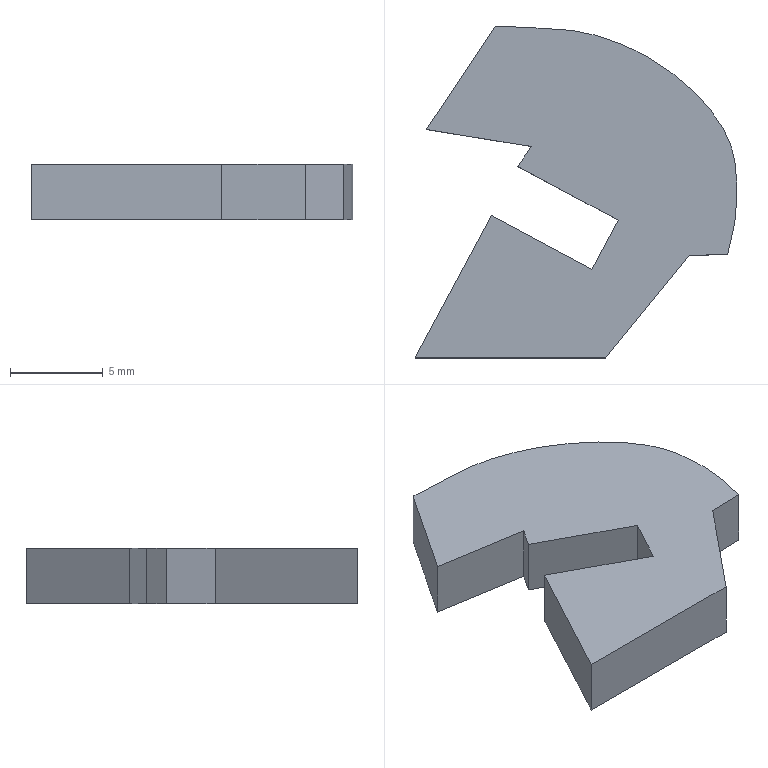Part | SolidWorks | features BaseBody 1 | 1 solid | 17 faces | box 17.352 x 17.888 x 3 mm | volume 573.183 mm3 | plane 13 | spline 4
STEP:
#1=CARTESIAN_POINT('',(42.678,-11.276,-1.5));
#2=VERTEX_POINT('',#1);
#3=CARTESIAN_POINT('',(42.678,-11.276,-1.5));
#4=VERTEX_POINT('',#3);
#5=CARTESIAN_POINT('',(42.678,-11.276,-1.5));
#6=CARTESIAN_POINT('',(42.678,-11.276,-1.5));
#7=CARTESIAN_POINT('',(42.678,-11.276,-1.5));
#8=CARTESIAN_POINT('',(42.678,-11.276,-1.5));
#9=B_SPLINE_CURVE_WITH_KNOTS('',3,(#5,#6,#7,#8),.UNSPECIFIED.,.F.,.F.,(4,4),(0.,0.000000418),.UNSPECIFIED.);
#10=EDGE_CURVE('',#2,#4,#9,.T.);
#11=ORIENTED_EDGE('',*,*,#10,.F.);
#12=CARTESIAN_POINT('',(40.608,-11.347,-1.5));
#13=VERTEX_POINT('',#12);
#14=CARTESIAN_POINT('',(42.678,-11.276,-1.5));
#15=DIRECTION('',(0.9994,0.03426,0.));
#16=VECTOR('',#15,1000.);
#17=LINE('',#14,#16);
#18=EDGE_CURVE('',#13,#2,#17,.T.);
#19=ORIENTED_EDGE('',*,*,#18,.F.);
#20=CARTESIAN_POINT('',(36.112,-16.862,-1.5));
#21=VERTEX_POINT('',#20);
#22=CARTESIAN_POINT('',(40.608,-11.347,-1.5));
#23=DIRECTION('',(0.6319,0.775,0.));
#24=VECTOR('',#23,1000.);
#25=LINE('',#22,#24);
#26=EDGE_CURVE('',#21,#13,#25,.T.);
#27=ORIENTED_EDGE('',*,*,#26,.F.);
#28=CARTESIAN_POINT('',(25.831,-16.862,-1.5));
#29=VERTEX_POINT('',#28);
#30=CARTESIAN_POINT('',(36.112,-16.862,-1.5));
#31=DIRECTION('',(1.,0.,0.));
#32=VECTOR('',#31,1000.);
#33=LINE('',#30,#32);
#34=EDGE_CURVE('',#29,#21,#33,.T.);
#35=ORIENTED_EDGE('',*,*,#34,.F.);
#36=CARTESIAN_POINT('',(29.948,-9.183,-1.5));
#37=VERTEX_POINT('',#36);
#38=CARTESIAN_POINT('',(25.831,-16.862,-1.5));
#39=DIRECTION('',(-0.4726,-0.8813,0.));
#40=VECTOR('',#39,1000.);
#41=LINE('',#38,#40);
#42=EDGE_CURVE('',#37,#29,#41,.T.);
#43=ORIENTED_EDGE('',*,*,#42,.F.);
#44=CARTESIAN_POINT('',(35.355,-12.082,-1.5));
#45=VERTEX_POINT('',#44);
#46=CARTESIAN_POINT('',(29.948,-9.183,-1.5));
#47=DIRECTION('',(-0.8814,0.4725,0.));
#48=VECTOR('',#47,1000.);
#49=LINE('',#46,#48);
#50=EDGE_CURVE('',#45,#37,#49,.T.);
#51=ORIENTED_EDGE('',*,*,#50,.F.);
#52=CARTESIAN_POINT('',(36.773,-9.438,-1.5));
#53=VERTEX_POINT('',#52);
#54=CARTESIAN_POINT('',(35.355,-12.082,-1.5));
#55=DIRECTION('',(-0.4725,-0.8814,0.));
#56=VECTOR('',#55,1000.);
#57=LINE('',#54,#56);
#58=EDGE_CURVE('',#53,#45,#57,.T.);
#59=ORIENTED_EDGE('',*,*,#58,.F.);
#60=CARTESIAN_POINT('',(31.367,-6.54,-1.5));
#61=VERTEX_POINT('',#60);
#62=CARTESIAN_POINT('',(36.773,-9.438,-1.5));
#63=DIRECTION('',(0.8814,-0.4725,0.));
#64=VECTOR('',#63,1000.);
#65=LINE('',#62,#64);
#66=EDGE_CURVE('',#61,#53,#65,.T.);
#67=ORIENTED_EDGE('',*,*,#66,.F.);
#68=CARTESIAN_POINT('',(32.093,-5.467,-1.5));
#69=VERTEX_POINT('',#68);
#70=CARTESIAN_POINT('',(31.367,-6.54,-1.5));
#71=DIRECTION('',(-0.5603,-0.8283,0.));
#72=VECTOR('',#71,1000.);
#73=LINE('',#70,#72);
#74=EDGE_CURVE('',#69,#61,#73,.T.);
#75=ORIENTED_EDGE('',*,*,#74,.F.);
#76=CARTESIAN_POINT('',(26.438,-4.552,-1.5));
#77=VERTEX_POINT('',#76);
#78=CARTESIAN_POINT('',(32.093,-5.467,-1.5));
#79=DIRECTION('',(0.9872,-0.1597,0.));
#80=VECTOR('',#79,1000.);
#81=LINE('',#78,#80);
#82=EDGE_CURVE('',#77,#69,#81,.T.);
#83=ORIENTED_EDGE('',*,*,#82,.F.);
#84=CARTESIAN_POINT('',(30.143,1.026,-1.5));
#85=VERTEX_POINT('',#84);
#86=CARTESIAN_POINT('',(26.438,-4.552,-1.5));
#87=DIRECTION('',(-0.5533,-0.833,0.));
#88=VECTOR('',#87,1000.);
#89=LINE('',#86,#88);
#90=EDGE_CURVE('',#85,#77,#89,.T.);
#91=ORIENTED_EDGE('',*,*,#90,.F.);
#92=CARTESIAN_POINT('',(30.208,1.022,-1.5));
#93=VERTEX_POINT('',#92);
#94=CARTESIAN_POINT('',(30.208,1.022,-1.5));
#95=CARTESIAN_POINT('',(30.186,1.023,-1.5));
#96=CARTESIAN_POINT('',(30.165,1.025,-1.5));
#97=CARTESIAN_POINT('',(30.143,1.026,-1.5));
#98=B_SPLINE_CURVE_WITH_KNOTS('',3,(#94,#95,#96,#97),.UNSPECIFIED.,.F.,.F.,(4,4),(0.08108,0.08126),.UNSPECIFIED.);
#99=EDGE_CURVE('',#93,#85,#98,.T.);
#100=ORIENTED_EDGE('',*,*,#99,.F.);
#101=CARTESIAN_POINT('',(36.936,0.04612,-1.5));
#102=VERTEX_POINT('',#101);
#103=CARTESIAN_POINT('',(36.936,0.04612,-1.5));
#104=CARTESIAN_POINT('',(34.519,1.041,-1.5));
#105=CARTESIAN_POINT('',(33.547,0.8089,-1.5));
#106=CARTESIAN_POINT('',(30.208,1.022,-1.5));
#107=B_SPLINE_CURVE_WITH_KNOTS('',3,(#103,#104,#105,#106),.UNSPECIFIED.,.F.,.F.,(4,4),(0.05405,0.08108),.UNSPECIFIED.);
#108=EDGE_CURVE('',#102,#93,#107,.T.);
#109=ORIENTED_EDGE('',*,*,#108,.F.);
#110=CARTESIAN_POINT('',(43.059,-6.232,-1.5));
#111=VERTEX_POINT('',#110);
#112=CARTESIAN_POINT('',(43.059,-6.232,-1.5));
#113=CARTESIAN_POINT('',(42.752,-3.979,-1.5));
#114=CARTESIAN_POINT('',(40.188,-1.29,-1.5));
#115=CARTESIAN_POINT('',(36.936,0.04612,-1.5));
#116=B_SPLINE_CURVE_WITH_KNOTS('',3,(#112,#113,#114,#115),.UNSPECIFIED.,.F.,.F.,(4,4),(0.02703,0.05405),.UNSPECIFIED.);
#117=EDGE_CURVE('',#111,#102,#116,.T.);
#118=ORIENTED_EDGE('',*,*,#117,.F.);
#119=CARTESIAN_POINT('',(42.678,-11.276,-1.5));
#120=CARTESIAN_POINT('',(43.027,-9.928,-1.5));
#121=CARTESIAN_POINT('',(43.376,-8.58,-1.5));
#122=CARTESIAN_POINT('',(43.059,-6.232,-1.5));
#123=B_SPLINE_CURVE_WITH_KNOTS('',3,(#119,#120,#121,#122),.UNSPECIFIED.,.F.,.F.,(4,4),(0.000000418,0.02703),.UNSPECIFIED.);
#124=EDGE_CURVE('',#4,#111,#123,.T.);
#125=ORIENTED_EDGE('',*,*,#124,.F.);
#126=EDGE_LOOP('',(#11,#19,#27,#35,#43,#51,#59,#67,#75,#83,#91,#100,#109,#118,#125));
#127=FACE_OUTER_BOUND('',#126,.T.);
#128=CARTESIAN_POINT('',(43.118,-9.129,-1.5));
#129=DIRECTION('',(0.,0.,-1.));
#130=DIRECTION('',(0.,-1.,0.));
#131=AXIS2_PLACEMENT_3D('',#128,#129,#130);
#132=PLANE('',#131);
#133=ADVANCED_FACE('',(#127),#132,.T.);
#134=CARTESIAN_POINT('',(42.678,-11.276,1.5));
#135=VERTEX_POINT('',#134);
#136=CARTESIAN_POINT('',(42.678,-11.276,1.5));
#137=VERTEX_POINT('',#136);
#138=CARTESIAN_POINT('',(42.678,-11.276,1.5));
#139=CARTESIAN_POINT('',(42.678,-11.276,1.5));
#140=CARTESIAN_POINT('',(42.678,-11.276,1.5));
#141=CARTESIAN_POINT('',(42.678,-11.276,1.5));
#142=B_SPLINE_CURVE_WITH_KNOTS('',3,(#138,#139,#140,#141),.UNSPECIFIED.,.F.,.F.,(4,4),(0.,0.000000418),.UNSPECIFIED.);
#143=EDGE_CURVE('',#135,#137,#142,.T.);
#144=ORIENTED_EDGE('',*,*,#143,.T.);
#145=CARTESIAN_POINT('',(43.059,-6.232,1.5));
#146=VERTEX_POINT('',#145);
#147=CARTESIAN_POINT('',(42.678,-11.276,1.5));
#148=CARTESIAN_POINT('',(43.027,-9.928,1.5));
#149=CARTESIAN_POINT('',(43.376,-8.58,1.5));
#150=CARTESIAN_POINT('',(43.059,-6.232,1.5));
#151=B_SPLINE_CURVE_WITH_KNOTS('',3,(#147,#148,#149,#150),.UNSPECIFIED.,.F.,.F.,(4,4),(0.000000418,0.02703),.UNSPECIFIED.);
#152=EDGE_CURVE('',#137,#146,#151,.T.);
#153=ORIENTED_EDGE('',*,*,#152,.T.);
#154=CARTESIAN_POINT('',(36.936,0.04612,1.5));
#155=VERTEX_POINT('',#154);
#156=CARTESIAN_POINT('',(43.059,-6.232,1.5));
#157=CARTESIAN_POINT('',(42.752,-3.979,1.5));
#158=CARTESIAN_POINT('',(40.188,-1.29,1.5));
#159=CARTESIAN_POINT('',(36.936,0.04612,1.5));
#160=B_SPLINE_CURVE_WITH_KNOTS('',3,(#156,#157,#158,#159),.UNSPECIFIED.,.F.,.F.,(4,4),(0.02703,0.05405),.UNSPECIFIED.);
#161=EDGE_CURVE('',#146,#155,#160,.T.);
#162=ORIENTED_EDGE('',*,*,#161,.T.);
#163=CARTESIAN_POINT('',(30.208,1.022,1.5));
#164=VERTEX_POINT('',#163);
#165=CARTESIAN_POINT('',(36.936,0.04612,1.5));
#166=CARTESIAN_POINT('',(34.519,1.041,1.5));
#167=CARTESIAN_POINT('',(33.547,0.8089,1.5));
#168=CARTESIAN_POINT('',(30.208,1.022,1.5));
#169=B_SPLINE_CURVE_WITH_KNOTS('',3,(#165,#166,#167,#168),.UNSPECIFIED.,.F.,.F.,(4,4),(0.05405,0.08108),.UNSPECIFIED.);
#170=EDGE_CURVE('',#155,#164,#169,.T.);
#171=ORIENTED_EDGE('',*,*,#170,.T.);
#172=CARTESIAN_POINT('',(30.143,1.026,1.5));
#173=VERTEX_POINT('',#172);
#174=CARTESIAN_POINT('',(30.208,1.022,1.5));
#175=CARTESIAN_POINT('',(30.186,1.023,1.5));
#176=CARTESIAN_POINT('',(30.165,1.025,1.5));
#177=CARTESIAN_POINT('',(30.143,1.026,1.5));
#178=B_SPLINE_CURVE_WITH_KNOTS('',3,(#174,#175,#176,#177),.UNSPECIFIED.,.F.,.F.,(4,4),(0.08108,0.08126),.UNSPECIFIED.);
#179=EDGE_CURVE('',#164,#173,#178,.T.);
#180=ORIENTED_EDGE('',*,*,#179,.T.);
#181=CARTESIAN_POINT('',(26.438,-4.552,1.5));
#182=VERTEX_POINT('',#181);
#183=CARTESIAN_POINT('',(26.438,-4.552,1.5));
#184=DIRECTION('',(-0.5533,-0.833,0.));
#185=VECTOR('',#184,1000.);
#186=LINE('',#183,#185);
#187=EDGE_CURVE('',#173,#182,#186,.T.);
#188=ORIENTED_EDGE('',*,*,#187,.T.);
#189=CARTESIAN_POINT('',(32.093,-5.467,1.5));
#190=VERTEX_POINT('',#189);
#191=CARTESIAN_POINT('',(32.093,-5.467,1.5));
#192=DIRECTION('',(0.9872,-0.1597,0.));
#193=VECTOR('',#192,1000.);
#194=LINE('',#191,#193);
#195=EDGE_CURVE('',#182,#190,#194,.T.);
#196=ORIENTED_EDGE('',*,*,#195,.T.);
#197=CARTESIAN_POINT('',(31.367,-6.54,1.5));
#198=VERTEX_POINT('',#197);
#199=CARTESIAN_POINT('',(31.367,-6.54,1.5));
#200=DIRECTION('',(-0.5603,-0.8283,0.));
#201=VECTOR('',#200,1000.);
#202=LINE('',#199,#201);
#203=EDGE_CURVE('',#190,#198,#202,.T.);
#204=ORIENTED_EDGE('',*,*,#203,.T.);
#205=CARTESIAN_POINT('',(36.773,-9.438,1.5));
#206=VERTEX_POINT('',#205);
#207=CARTESIAN_POINT('',(36.773,-9.438,1.5));
#208=DIRECTION('',(0.8814,-0.4725,0.));
#209=VECTOR('',#208,1000.);
#210=LINE('',#207,#209);
#211=EDGE_CURVE('',#198,#206,#210,.T.);
#212=ORIENTED_EDGE('',*,*,#211,.T.);
#213=CARTESIAN_POINT('',(35.355,-12.082,1.5));
#214=VERTEX_POINT('',#213);
#215=CARTESIAN_POINT('',(35.355,-12.082,1.5));
#216=DIRECTION('',(-0.4725,-0.8814,0.));
#217=VECTOR('',#216,1000.);
#218=LINE('',#215,#217);
#219=EDGE_CURVE('',#206,#214,#218,.T.);
#220=ORIENTED_EDGE('',*,*,#219,.T.);
#221=CARTESIAN_POINT('',(29.948,-9.183,1.5));
#222=VERTEX_POINT('',#221);
#223=CARTESIAN_POINT('',(29.948,-9.183,1.5));
#224=DIRECTION('',(-0.8814,0.4725,0.));
#225=VECTOR('',#224,1000.);
#226=LINE('',#223,#225);
#227=EDGE_CURVE('',#214,#222,#226,.T.);
#228=ORIENTED_EDGE('',*,*,#227,.T.);
#229=CARTESIAN_POINT('',(25.831,-16.862,1.5));
#230=VERTEX_POINT('',#229);
#231=CARTESIAN_POINT('',(25.831,-16.862,1.5));
#232=DIRECTION('',(-0.4726,-0.8813,0.));
#233=VECTOR('',#232,1000.);
#234=LINE('',#231,#233);
#235=EDGE_CURVE('',#222,#230,#234,.T.);
#236=ORIENTED_EDGE('',*,*,#235,.T.);
#237=CARTESIAN_POINT('',(36.112,-16.862,1.5));
#238=VERTEX_POINT('',#237);
#239=CARTESIAN_POINT('',(36.112,-16.862,1.5));
#240=DIRECTION('',(1.,0.,0.));
#241=VECTOR('',#240,1000.);
#242=LINE('',#239,#241);
#243=EDGE_CURVE('',#230,#238,#242,.T.);
#244=ORIENTED_EDGE('',*,*,#243,.T.);
#245=CARTESIAN_POINT('',(40.608,-11.347,1.5));
#246=VERTEX_POINT('',#245);
#247=CARTESIAN_POINT('',(40.608,-11.347,1.5));
#248=DIRECTION('',(0.6319,0.775,0.));
#249=VECTOR('',#248,1000.);
#250=LINE('',#247,#249);
#251=EDGE_CURVE('',#238,#246,#250,.T.);
#252=ORIENTED_EDGE('',*,*,#251,.T.);
#253=CARTESIAN_POINT('',(42.678,-11.276,1.5));
#254=DIRECTION('',(0.9994,0.03426,0.));
#255=VECTOR('',#254,1000.);
#256=LINE('',#253,#255);
#257=EDGE_CURVE('',#246,#135,#256,.T.);
#258=ORIENTED_EDGE('',*,*,#257,.T.);
#259=EDGE_LOOP('',(#144,#153,#162,#171,#180,#188,#196,#204,#212,#220,#228,#236,#244,#252,#258));
#260=FACE_OUTER_BOUND('',#259,.T.);
#261=CARTESIAN_POINT('',(43.118,-9.129,1.5));
#262=DIRECTION('',(0.,0.,-1.));
#263=DIRECTION('',(0.,-1.,0.));
#264=AXIS2_PLACEMENT_3D('',#261,#262,#263);
#265=PLANE('',#264);
#266=ADVANCED_FACE('',(#260),#265,.F.);
#267=ORIENTED_EDGE('',*,*,#18,.T.);
#268=CARTESIAN_POINT('',(42.678,-11.276,1.5));
#269=DIRECTION('',(0.,0.,-1.));
#270=VECTOR('',#269,1000.);
#271=LINE('',#268,#270);
#272=EDGE_CURVE('',#135,#2,#271,.T.);
#273=ORIENTED_EDGE('',*,*,#272,.F.);
#274=ORIENTED_EDGE('',*,*,#257,.F.);
#275=CARTESIAN_POINT('',(40.608,-11.347,1.5));
#276=DIRECTION('',(0.,0.,-1.));
#277=VECTOR('',#276,1000.);
#278=LINE('',#275,#277);
#279=EDGE_CURVE('',#246,#13,#278,.T.);
#280=ORIENTED_EDGE('',*,*,#279,.T.);
#281=EDGE_LOOP('',(#267,#273,#274,#280));
#282=FACE_OUTER_BOUND('',#281,.T.);
#283=CARTESIAN_POINT('',(42.678,-11.276,1.5));
#284=DIRECTION('',(-0.03426,0.9994,0.));
#285=DIRECTION('',(0.,0.,1.));
#286=AXIS2_PLACEMENT_3D('',#283,#284,#285);
#287=PLANE('',#286);
#288=ADVANCED_FACE('',(#282),#287,.F.);
#289=ORIENTED_EDGE('',*,*,#26,.T.);
#290=ORIENTED_EDGE('',*,*,#279,.F.);
#291=ORIENTED_EDGE('',*,*,#251,.F.);
#292=CARTESIAN_POINT('',(36.112,-16.862,1.5));
#293=DIRECTION('',(0.,0.,-1.));
#294=VECTOR('',#293,1000.);
#295=LINE('',#292,#294);
#296=EDGE_CURVE('',#238,#21,#295,.T.);
#297=ORIENTED_EDGE('',*,*,#296,.T.);
#298=EDGE_LOOP('',(#289,#290,#291,#297));
#299=FACE_OUTER_BOUND('',#298,.T.);
#300=CARTESIAN_POINT('',(40.608,-11.347,1.5));
#301=DIRECTION('',(-0.775,0.6319,0.));
#302=DIRECTION('',(0.,0.,1.));
#303=AXIS2_PLACEMENT_3D('',#300,#301,#302);
#304=PLANE('',#303);
#305=ADVANCED_FACE('',(#299),#304,.F.);
#306=ORIENTED_EDGE('',*,*,#34,.T.);
#307=ORIENTED_EDGE('',*,*,#296,.F.);
#308=ORIENTED_EDGE('',*,*,#243,.F.);
#309=CARTESIAN_POINT('',(25.831,-16.862,1.5));
#310=DIRECTION('',(0.,0.,-1.));
#311=VECTOR('',#310,1000.);
#312=LINE('',#309,#311);
#313=EDGE_CURVE('',#230,#29,#312,.T.);
#314=ORIENTED_EDGE('',*,*,#313,.T.);
#315=EDGE_LOOP('',(#306,#307,#308,#314));
#316=FACE_OUTER_BOUND('',#315,.T.);
#317=CARTESIAN_POINT('',(36.112,-16.862,1.5));
#318=DIRECTION('',(0.,1.,0.));
#319=DIRECTION('',(1.,0.,0.));
#320=AXIS2_PLACEMENT_3D('',#317,#318,#319);
#321=PLANE('',#320);
#322=ADVANCED_FACE('',(#316),#321,.F.);
#323=ORIENTED_EDGE('',*,*,#42,.T.);
#324=ORIENTED_EDGE('',*,*,#313,.F.);
#325=ORIENTED_EDGE('',*,*,#235,.F.);
#326=CARTESIAN_POINT('',(29.948,-9.183,1.5));
#327=DIRECTION('',(0.,0.,-1.));
#328=VECTOR('',#327,1000.);
#329=LINE('',#326,#328);
#330=EDGE_CURVE('',#222,#37,#329,.T.);
#331=ORIENTED_EDGE('',*,*,#330,.T.);
#332=EDGE_LOOP('',(#323,#324,#325,#331));
#333=FACE_OUTER_BOUND('',#332,.T.);
#334=CARTESIAN_POINT('',(25.831,-16.862,1.5));
#335=DIRECTION('',(0.8813,-0.4726,0.));
#336=DIRECTION('',(0.,0.,-1.));
#337=AXIS2_PLACEMENT_3D('',#334,#335,#336);
#338=PLANE('',#337);
#339=ADVANCED_FACE('',(#333),#338,.F.);
#340=ORIENTED_EDGE('',*,*,#50,.T.);
#341=ORIENTED_EDGE('',*,*,#330,.F.);
#342=ORIENTED_EDGE('',*,*,#227,.F.);
#343=CARTESIAN_POINT('',(35.355,-12.082,1.5));
#344=DIRECTION('',(0.,0.,-1.));
#345=VECTOR('',#344,1000.);
#346=LINE('',#343,#345);
#347=EDGE_CURVE('',#214,#45,#346,.T.);
#348=ORIENTED_EDGE('',*,*,#347,.T.);
#349=EDGE_LOOP('',(#340,#341,#342,#348));
#350=FACE_OUTER_BOUND('',#349,.T.);
#351=CARTESIAN_POINT('',(29.948,-9.183,1.5));
#352=DIRECTION('',(-0.4725,-0.8814,0.));
#353=DIRECTION('',(-0.8814,0.4725,0.));
#354=AXIS2_PLACEMENT_3D('',#351,#352,#353);
#355=PLANE('',#354);
#356=ADVANCED_FACE('',(#350),#355,.F.);
#357=ORIENTED_EDGE('',*,*,#58,.T.);
#358=ORIENTED_EDGE('',*,*,#347,.F.);
#359=ORIENTED_EDGE('',*,*,#219,.F.);
#360=CARTESIAN_POINT('',(36.773,-9.438,1.5));
#361=DIRECTION('',(0.,0.,-1.));
#362=VECTOR('',#361,1000.);
#363=LINE('',#360,#362);
#364=EDGE_CURVE('',#206,#53,#363,.T.);
#365=ORIENTED_EDGE('',*,*,#364,.T.);
#366=EDGE_LOOP('',(#357,#358,#359,#365));
#367=FACE_OUTER_BOUND('',#366,.T.);
#368=CARTESIAN_POINT('',(35.355,-12.082,1.5));
#369=DIRECTION('',(0.8814,-0.4725,0.));
#370=DIRECTION('',(0.,0.,-1.));
#371=AXIS2_PLACEMENT_3D('',#368,#369,#370);
#372=PLANE('',#371);
#373=ADVANCED_FACE('',(#367),#372,.F.);
#374=ORIENTED_EDGE('',*,*,#66,.T.);
#375=ORIENTED_EDGE('',*,*,#364,.F.);
#376=ORIENTED_EDGE('',*,*,#211,.F.);
#377=CARTESIAN_POINT('',(31.367,-6.54,1.5));
#378=DIRECTION('',(0.,0.,-1.));
#379=VECTOR('',#378,1000.);
#380=LINE('',#377,#379);
#381=EDGE_CURVE('',#198,#61,#380,.T.);
#382=ORIENTED_EDGE('',*,*,#381,.T.);
#383=EDGE_LOOP('',(#374,#375,#376,#382));
#384=FACE_OUTER_BOUND('',#383,.T.);
#385=CARTESIAN_POINT('',(36.773,-9.438,1.5));
#386=DIRECTION('',(0.4725,0.8814,0.));
#387=DIRECTION('',(0.,0.,-1.));
#388=AXIS2_PLACEMENT_3D('',#385,#386,#387);
#389=PLANE('',#388);
#390=ADVANCED_FACE('',(#384),#389,.F.);
#391=ORIENTED_EDGE('',*,*,#74,.T.);
#392=ORIENTED_EDGE('',*,*,#381,.F.);
#393=ORIENTED_EDGE('',*,*,#203,.F.);
#394=CARTESIAN_POINT('',(32.093,-5.467,1.5));
#395=DIRECTION('',(0.,0.,-1.));
#396=VECTOR('',#395,1000.);
#397=LINE('',#394,#396);
#398=EDGE_CURVE('',#190,#69,#397,.T.);
#399=ORIENTED_EDGE('',*,*,#398,.T.);
#400=EDGE_LOOP('',(#391,#392,#393,#399));
#401=FACE_OUTER_BOUND('',#400,.T.);
#402=CARTESIAN_POINT('',(31.367,-6.54,1.5));
#403=DIRECTION('',(0.8283,-0.5603,0.));
#404=DIRECTION('',(0.,0.,-1.));
#405=AXIS2_PLACEMENT_3D('',#402,#403,#404);
#406=PLANE('',#405);
#407=ADVANCED_FACE('',(#401),#406,.F.);
#408=ORIENTED_EDGE('',*,*,#82,.T.);
#409=ORIENTED_EDGE('',*,*,#398,.F.);
#410=ORIENTED_EDGE('',*,*,#195,.F.);
#411=CARTESIAN_POINT('',(26.438,-4.552,1.5));
#412=DIRECTION('',(0.,0.,-1.));
#413=VECTOR('',#412,1000.);
#414=LINE('',#411,#413);
#415=EDGE_CURVE('',#182,#77,#414,.T.);
#416=ORIENTED_EDGE('',*,*,#415,.T.);
#417=EDGE_LOOP('',(#408,#409,#410,#416));
#418=FACE_OUTER_BOUND('',#417,.T.);
#419=CARTESIAN_POINT('',(32.093,-5.467,1.5));
#420=DIRECTION('',(0.1597,0.9872,0.));
#421=DIRECTION('',(0.,0.,-1.));
#422=AXIS2_PLACEMENT_3D('',#419,#420,#421);
#423=PLANE('',#422);
#424=ADVANCED_FACE('',(#418),#423,.F.);
#425=ORIENTED_EDGE('',*,*,#90,.T.);
#426=ORIENTED_EDGE('',*,*,#415,.F.);
#427=ORIENTED_EDGE('',*,*,#187,.F.);
#428=CARTESIAN_POINT('',(30.143,1.026,1.5));
#429=DIRECTION('',(0.,0.,-1.));
#430=VECTOR('',#429,1000.);
#431=LINE('',#428,#430);
#432=EDGE_CURVE('',#173,#85,#431,.T.);
#433=ORIENTED_EDGE('',*,*,#432,.T.);
#434=EDGE_LOOP('',(#425,#426,#427,#433));
#435=FACE_OUTER_BOUND('',#434,.T.);
#436=CARTESIAN_POINT('',(26.438,-4.552,1.5));
#437=DIRECTION('',(0.833,-0.5533,0.));
#438=DIRECTION('',(0.,0.,-1.));
#439=AXIS2_PLACEMENT_3D('',#436,#437,#438);
#440=PLANE('',#439);
#441=ADVANCED_FACE('',(#435),#440,.F.);
#442=ORIENTED_EDGE('',*,*,#99,.T.);
#443=ORIENTED_EDGE('',*,*,#432,.F.);
#444=ORIENTED_EDGE('',*,*,#179,.F.);
#445=CARTESIAN_POINT('',(30.208,1.022,1.5));
#446=DIRECTION('',(0.,0.,-1.));
#447=VECTOR('',#446,1000.);
#448=LINE('',#445,#447);
#449=EDGE_CURVE('',#164,#93,#448,.T.);
#450=ORIENTED_EDGE('',*,*,#449,.T.);
#451=EDGE_LOOP('',(#442,#443,#444,#450));
#452=FACE_OUTER_BOUND('',#451,.T.);
#453=CARTESIAN_POINT('',(30.208,1.022,1.5));
#454=CARTESIAN_POINT('',(30.208,1.022,-1.5));
#455=CARTESIAN_POINT('',(30.186,1.023,1.5));
#456=CARTESIAN_POINT('',(30.186,1.023,-1.5));
#457=CARTESIAN_POINT('',(30.165,1.025,1.5));
#458=CARTESIAN_POINT('',(30.165,1.025,-1.5));
#459=CARTESIAN_POINT('',(30.143,1.026,1.5));
#460=CARTESIAN_POINT('',(30.143,1.026,-1.5));
#461=B_SPLINE_SURFACE_WITH_KNOTS('',3,1,((#453,#454),(#455,#456),(#457,#458),(#459,#460)),.UNSPECIFIED.,.F.,.F.,.F.,(4,4),(2,2),(0.08108,0.08126),(0.,1.),.UNSPECIFIED.);
#462=ADVANCED_FACE('',(#452),#461,.F.);
#463=ORIENTED_EDGE('',*,*,#108,.T.);
#464=ORIENTED_EDGE('',*,*,#449,.F.);
#465=ORIENTED_EDGE('',*,*,#170,.F.);
#466=CARTESIAN_POINT('',(36.936,0.04612,1.5));
#467=DIRECTION('',(0.,0.,-1.));
#468=VECTOR('',#467,1000.);
#469=LINE('',#466,#468);
#470=EDGE_CURVE('',#155,#102,#469,.T.);
#471=ORIENTED_EDGE('',*,*,#470,.T.);
#472=EDGE_LOOP('',(#463,#464,#465,#471));
#473=FACE_OUTER_BOUND('',#472,.T.);
#474=CARTESIAN_POINT('',(36.936,0.04612,1.5));
#475=CARTESIAN_POINT('',(36.936,0.04612,-1.5));
#476=CARTESIAN_POINT('',(34.519,1.041,1.5));
#477=CARTESIAN_POINT('',(34.519,1.041,-1.5));
#478=CARTESIAN_POINT('',(33.547,0.8089,1.5));
#479=CARTESIAN_POINT('',(33.547,0.8089,-1.5));
#480=CARTESIAN_POINT('',(30.208,1.022,1.5));
#481=CARTESIAN_POINT('',(30.208,1.022,-1.5));
#482=B_SPLINE_SURFACE_WITH_KNOTS('',3,1,((#474,#475),(#476,#477),(#478,#479),(#480,#481)),.UNSPECIFIED.,.F.,.F.,.F.,(4,4),(2,2),(0.05405,0.08108),(0.,1.),.UNSPECIFIED.);
#483=ADVANCED_FACE('',(#473),#482,.F.);
#484=ORIENTED_EDGE('',*,*,#117,.T.);
#485=ORIENTED_EDGE('',*,*,#470,.F.);
#486=ORIENTED_EDGE('',*,*,#161,.F.);
#487=CARTESIAN_POINT('',(43.059,-6.232,1.5));
#488=DIRECTION('',(0.,0.,-1.));
#489=VECTOR('',#488,1000.);
#490=LINE('',#487,#489);
#491=EDGE_CURVE('',#146,#111,#490,.T.);
#492=ORIENTED_EDGE('',*,*,#491,.T.);
#493=EDGE_LOOP('',(#484,#485,#486,#492));
#494=FACE_OUTER_BOUND('',#493,.T.);
#495=CARTESIAN_POINT('',(43.059,-6.232,1.5));
#496=CARTESIAN_POINT('',(43.059,-6.232,-1.5));
#497=CARTESIAN_POINT('',(42.752,-3.979,1.5));
#498=CARTESIAN_POINT('',(42.752,-3.979,-1.5));
#499=CARTESIAN_POINT('',(40.188,-1.29,1.5));
#500=CARTESIAN_POINT('',(40.188,-1.29,-1.5));
#501=CARTESIAN_POINT('',(36.936,0.04612,1.5));
#502=CARTESIAN_POINT('',(36.936,0.04612,-1.5));
#503=B_SPLINE_SURFACE_WITH_KNOTS('',3,1,((#495,#496),(#497,#498),(#499,#500),(#501,#502)),.UNSPECIFIED.,.F.,.F.,.F.,(4,4),(2,2),(0.02703,0.05405),(0.,1.),.UNSPECIFIED.);
#504=ADVANCED_FACE('',(#494),#503,.F.);
#505=ORIENTED_EDGE('',*,*,#124,.T.);
#506=ORIENTED_EDGE('',*,*,#491,.F.);
#507=ORIENTED_EDGE('',*,*,#152,.F.);
#508=CARTESIAN_POINT('',(42.678,-11.276,1.5));
#509=DIRECTION('',(0.,0.,-1.));
#510=VECTOR('',#509,1000.);
#511=LINE('',#508,#510);
#512=EDGE_CURVE('',#137,#4,#511,.T.);
#513=ORIENTED_EDGE('',*,*,#512,.T.);
#514=EDGE_LOOP('',(#505,#506,#507,#513));
#515=FACE_OUTER_BOUND('',#514,.T.);
#516=CARTESIAN_POINT('',(42.678,-11.276,1.5));
#517=CARTESIAN_POINT('',(42.678,-11.276,-1.5));
#518=CARTESIAN_POINT('',(43.027,-9.928,1.5));
#519=CARTESIAN_POINT('',(43.027,-9.928,-1.5));
#520=CARTESIAN_POINT('',(43.376,-8.58,1.5));
#521=CARTESIAN_POINT('',(43.376,-8.58,-1.5));
#522=CARTESIAN_POINT('',(43.059,-6.232,1.5));
#523=CARTESIAN_POINT('',(43.059,-6.232,-1.5));
#524=B_SPLINE_SURFACE_WITH_KNOTS('',3,1,((#516,#517),(#518,#519),(#520,#521),(#522,#523)),.UNSPECIFIED.,.F.,.F.,.F.,(4,4),(2,2),(0.000000418,0.02703),(0.,1.),.UNSPECIFIED.);
#525=ADVANCED_FACE('',(#515),#524,.F.);
#526=ORIENTED_EDGE('',*,*,#10,.T.);
#527=ORIENTED_EDGE('',*,*,#512,.F.);
#528=ORIENTED_EDGE('',*,*,#143,.F.);
#529=ORIENTED_EDGE('',*,*,#272,.T.);
#530=EDGE_LOOP('',(#526,#527,#528,#529));
#531=FACE_OUTER_BOUND('',#530,.T.);
#532=CARTESIAN_POINT('',(42.678,-11.276,1.5));
#533=DIRECTION('',(-0.968,0.251,0.));
#534=DIRECTION('',(0.,0.,1.));
#535=AXIS2_PLACEMENT_3D('',#532,#533,#534);
#536=PLANE('',#535);
#537=ADVANCED_FACE('',(#531),#536,.F.);
#538=CLOSED_SHELL('',(#133,#266,#288,#305,#322,#339,#356,#373,#390,#407,#424,#441,#462,#483,#504,#525,#537));
#539=MANIFOLD_SOLID_BREP('',#538);
#540=CARTESIAN_POINT('',(0.,0.,0.));
#541=DIRECTION('',(0.,0.,1.));
#542=DIRECTION('',(1.,0.,0.));
#543=AXIS2_PLACEMENT_3D('',#540,#541,#542);
#544=(LENGTH_UNIT()NAMED_UNIT(*)SI_UNIT(.MILLI.,.METRE.));
#545=UNCERTAINTY_MEASURE_WITH_UNIT(LENGTH_MEASURE(0.00001),#544,'','');
#546=(NAMED_UNIT(*)PLANE_ANGLE_UNIT()SI_UNIT($,.RADIAN.));
#547=(NAMED_UNIT(*)SI_UNIT($,.STERADIAN.)SOLID_ANGLE_UNIT());
#548=(GEOMETRIC_REPRESENTATION_CONTEXT(3)GLOBAL_UNCERTAINTY_ASSIGNED_CONTEXT((#545))GLOBAL_UNIT_ASSIGNED_CONTEXT((#544,#546,#547))REPRESENTATION_CONTEXT('',''));
#549=ADVANCED_BREP_SHAPE_REPRESENTATION('',(#539,#543),#548);